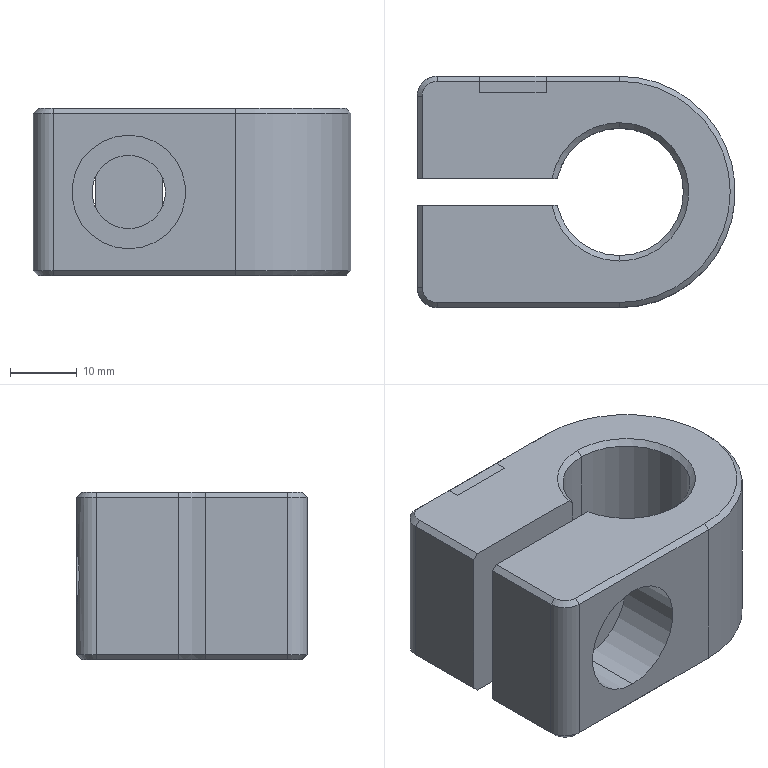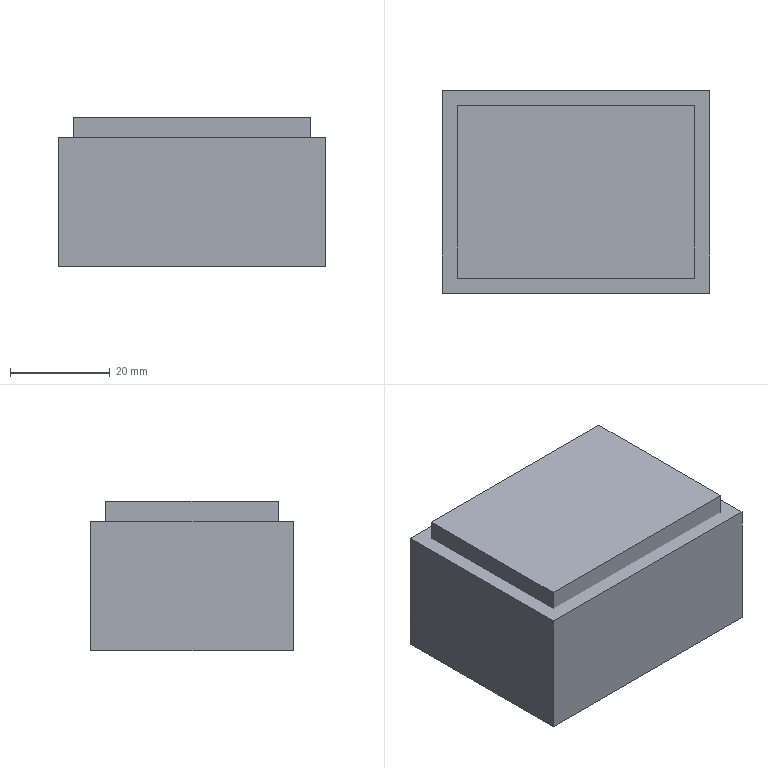CAM job | NX | 3+2 milling, drilling | part box 47.6 x 34.6 x 25 mm | stock box 53.6 x 40.6 x 30 mm
Tools:
number,name,description,diameter,corner_radius,flute_length,length,flutes
1,D63,Milling Tool-5 Parameters,63.0,0.0,50.0,75.0,2
10,D10,Milling Tool-5 Parameters,10.0,0.0,50.0,75.0,2
11,D10JING,Milling Tool-5 Parameters,10.0,0.0,50.0,75.0,2
7,D6A45,Milling Tool-5 Parameters,6.0,0.0,3.0,3.0,2
12,11.0ZT,Drilling Tool,11.0,0.0,35.0,50.0,2
6,D6,Milling Tool-5 Parameters,6.0,0.0,50.0,75.0,2
4,D4,Milling Tool-5 Parameters,4.0,0.0,50.0,75.0,2
13,T110H4,Milling Tool-T Cutter,110.0,,4.0,25.0,4
Operations:
program,operation,operation_type,tool,method,geometry_group,spindle_rpm,surface_speed,feed_per_tooth,feed_cut,feed_plunge,cut_length_mm,path_length_mm,cut_time_min,machine_time_min
1-50X35X30毛胚-G54G55,FLOOR_WALL,VolumeBased25DMillingOperation,D63,METHOD,A,6500.0,1286.0,0.0962,1250.0,100.0,128.6,182.6,0.1029,0.1083
1-50X35X30毛胚-G54G55,FLOOR_WALL_COPY_1,VolumeBased25DMillingOperation,D63,METHOD,AA,6500.0,1286.0,0.0962,1250.0,100.0,128.6,182.6,0.1029,0.1083
1-50X35X30毛胚-G54G55,ADAPTIVE_MILLING,CavityMilling,D10,METHOD,A,8000.0,251.0,0.2188,3500.0,1000.0,4013.196,4441.588,2.42,2.463
1-50X35X30毛胚-G54G55,ADAPTIVE_MILLING_COPY,CavityMilling,D10,METHOD,AA,8000.0,251.0,0.2188,3500.0,1000.0,4013.196,4441.588,2.42,2.463
1-50X35X30毛胚-G54G55,ZLEVEL_PROFILE_COPY_COPY_1,ZLevelMilling,D10JING,METHOD,A,8000.0,251.0,0.05,800.0,100.0,441.473,678.673,0.5518,0.5756
1-50X35X30毛胚-G54G55,ZLEVEL_PROFILE_COPY_COPY_1_COPY_1,ZLevelMilling,D10JING,METHOD,AA,8000.0,251.0,0.05,800.0,100.0,441.473,678.673,0.5518,0.5756
1-50X35X30毛胚-G54G55,ZLEVEL_PROFILE_1_COPY_1_COPY_COPY_1_COPY,ZLevelMilling,D6A45,METHOD,A,7500.0,141.0,0.0667,1000.0,100.0,218.032,367.766,0.218,0.233
1-50X35X30毛胚-G54G55,ZLEVEL_PROFILE_1_COPY_1_COPY_COPY_1_COPY_COPY_1,ZLevelMilling,D6A45,METHOD,AA,7500.0,141.0,0.0667,1000.0,100.0,218.032,367.766,0.218,0.233
2-50X35X30毛胚-G54G55,FLOOR_WALL_COPY,VolumeBased25DMillingOperation,D63,METHOD,B,6500.0,1286.0,0.0962,1250.0,100.0,613.0,1329.401,0.4904,0.562
2-50X35X30毛胚-G54G55,FLOOR_WALL_COPY_COPY,VolumeBased25DMillingOperation,D63,METHOD,BB,6500.0,1286.0,0.0962,1250.0,100.0,613.0,1329.401,0.4904,0.562
2-50X35X30毛胚-G54G55,ZLEVEL_PROFILE_1_COPY_1_COPY_COPY_1_COPY_COPY,ZLevelMilling,D6A45,METHOD,B,7500.0,141.0,0.0667,1000.0,100.0,218.032,367.767,0.218,0.233
2-50X35X30毛胚-G54G55,ZLEVEL_PROFILE_1_COPY_1_COPY_COPY_1_COPY_COPY_COPY_1,ZLevelMilling,D6A45,METHOD,BB,7500.0,141.0,0.0667,1000.0,100.0,218.032,367.767,0.218,0.233
3-50X35X30毛胚-G54G55,DRILLING_COPY_1,Operation,D6A45,METHOD,C,3000.0,56.0,0.0333,200.0,0.0,4.0,68.0,0.02,0.0264
3-50X35X30毛胚-G54G55,DRILLING_COPY_1_COPY,Operation,D6A45,METHOD,CC,3000.0,56.0,0.0333,200.0,0.0,4.0,68.0,0.02,0.0264
3-50X35X30毛胚-G54G55,DRILLING_COPY_1_COPY_COPY,Operation,11.0ZT,METHOD,C,1500.0,55.0,0.0667,200.0,0.0,41.305,142.609,0.2065,0.2167
3-50X35X30毛胚-G54G55,DRILLING_COPY_1_COPY_COPY_COPY,Operation,11.0ZT,METHOD,CC,1500.0,55.0,0.0667,200.0,0.0,41.305,142.609,0.2065,0.2167
3-50X35X30毛胚-G54G55,ZLEVEL_PROFILE_COPY_COPY_1_COPY,ZLevelMilling,D10JING,METHOD,C,8000.0,251.0,0.1,1600.0,100.0,285.921,352.921,0.1787,0.1854
3-50X35X30毛胚-G54G55,ZLEVEL_PROFILE_COPY_COPY_1_COPY_COPY,ZLevelMilling,D10JING,METHOD,CC,8000.0,251.0,0.1,1600.0,100.0,285.921,352.921,0.1787,0.1854
3-50X35X30毛胚-G54G55,ZLEVEL_PROFILE_1_COPY_1_COPY_COPY_1_COPY_COPY_COPY,ZLevelMilling,D6A45,METHOD,C,7500.0,141.0,0.0667,1000.0,100.0,52.68,112.68,0.0527,0.0587
3-50X35X30毛胚-G54G55,ZLEVEL_PROFILE_1_COPY_1_COPY_COPY_1_COPY_COPY_COPY_COPY_1,ZLevelMilling,D6A45,METHOD,CC,7500.0,141.0,0.0667,1000.0,100.0,52.68,112.68,0.0527,0.0587
4-50X35X30毛胚-G54G55,FLOOR_WALL_1,VolumeBased25DMillingOperation,D6,METHOD,D,8000.0,150.0,0.1562,2500.0,1000.0,780.136,910.282,0.3304,0.3434
4-50X35X30毛胚-G54G55,FLOOR_WALL_1_COPY,VolumeBased25DMillingOperation,D6,METHOD,DD,8000.0,150.0,0.1562,2500.0,1000.0,780.136,910.282,0.3304,0.3434
4-50X35X30毛胚-G54G55,DRILLING_COPY_1_COPY_1,Operation,D6A45,METHOD,D,3000.0,56.0,0.0333,200.0,0.0,4.0,73.0,0.02,0.0269
4-50X35X30毛胚-G54G55,DRILLING_COPY_1_COPY_1_COPY,Operation,D6A45,METHOD,DD,3000.0,56.0,0.0333,200.0,0.0,4.0,73.0,0.02,0.0269
4-50X35X30毛胚-G54G55,DRILLING_COPY_1_COPY_COPY_COPY_1,Operation,11.0ZT,METHOD,D,1500.0,55.0,0.0667,200.0,0.0,39.305,143.609,0.1965,0.207
4-50X35X30毛胚-G54G55,DRILLING_COPY_1_COPY_COPY_COPY_1_COPY,Operation,11.0ZT,METHOD,DD,1500.0,55.0,0.0667,200.0,0.0,39.305,143.609,0.1965,0.207
4-50X35X30毛胚-G54G55,ZLEVEL_PROFILE_COPY_1_COPY_1_COPY_1_1_COPY_COPY_COPY_1,ZLevelMilling,D4,METHOD,D,7000.0,87.0,0.1071,1500.0,800.0,515.329,733.458,0.3758,0.3976
4-50X35X30毛胚-G54G55,FLOOR_WALL_1_1_COPY_COPY_1,VolumeBased25DMillingOperation,D4,METHOD,D,7000.0,219.0,0.0893,1250.0,100.0,376.202,579.225,0.301,0.3213
4-50X35X30毛胚-G54G55,ZLEVEL_PROFILE_COPY_1_COPY_1_COPY_1_1_COPY_COPY_COPY_1_COPY,ZLevelMilling,D4,METHOD,DD,7000.0,87.0,0.1071,1500.0,800.0,515.329,733.458,0.3758,0.3976
4-50X35X30毛胚-G54G55,FLOOR_WALL_1_1_COPY_COPY_1_COPY,VolumeBased25DMillingOperation,D4,METHOD,DD,7000.0,219.0,0.0893,1250.0,100.0,376.202,579.225,0.301,0.3213
4-50X35X30毛胚-G54G55,ZLEVEL_PROFILE_1_COPY_1_COPY_COPY_1_COPY_COPY_COPY_COPY,ZLevelMilling,D6A45,METHOD,D,7500.0,141.0,0.0667,1000.0,100.0,103.547,311.242,0.1035,0.1243
4-50X35X30毛胚-G54G55,ZLEVEL_PROFILE_1_COPY_1_COPY_COPY_1_COPY_COPY_COPY_COPY_COPY,ZLevelMilling,D6A45,METHOD,D,7500.0,141.0,0.0667,1000.0,100.0,34.349,99.349,0.0343,0.0408
4-50X35X30毛胚-G54G55,ZLEVEL_PROFILE_1_COPY_1_COPY_COPY_1_COPY_COPY_COPY_COPY_COPY_1,ZLevelMilling,D6A45,METHOD,DD,7500.0,141.0,0.0667,1000.0,100.0,103.547,311.242,0.1035,0.1243
4-50X35X30毛胚-G54G55,ZLEVEL_PROFILE_1_COPY_1_COPY_COPY_1_COPY_COPY_COPY_COPY_COPY_COPY,ZLevelMilling,D6A45,METHOD,DD,7500.0,141.0,0.0667,1000.0,100.0,34.349,99.349,0.0343,0.0408
4-50X35X30毛胚-G54G55,PLANAR_MILL,PlanarMilling,T110H4,METHOD,D,4000.0,1382.0,0.0219,350.0,100.0,161.4,254.0,0.4611,0.4704
4-50X35X30毛胚-G54G55,PLANAR_MILL_COPY,PlanarMilling,T110H4,METHOD,DD,4000.0,1382.0,0.0219,350.0,100.0,161.4,254.0,0.4611,0.4704